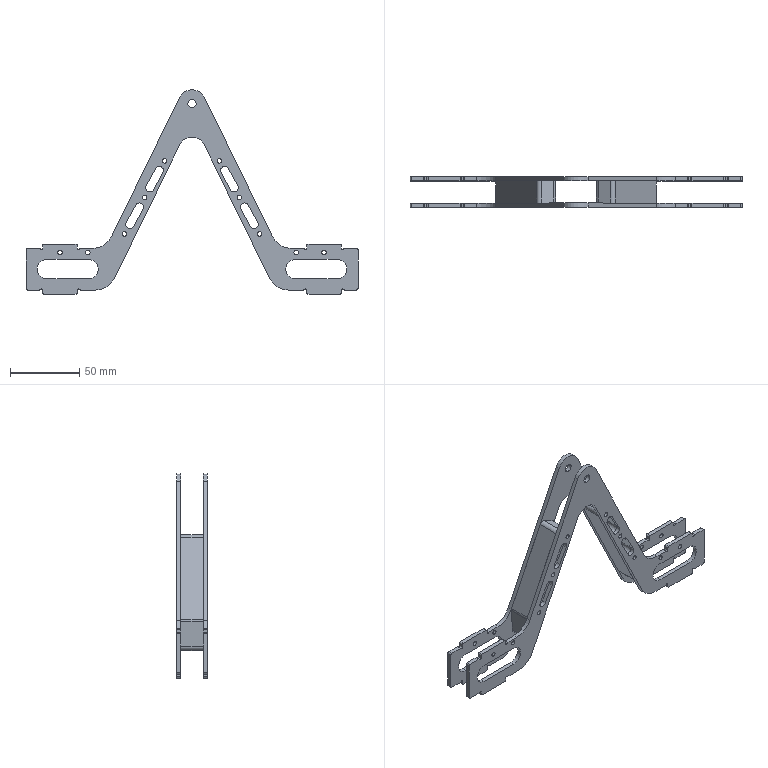Part | SolidWorks | features ICE 5, Extrusion 1, Fillet 1, MirrorSolid 1 | 4 solids | 286 faces | box 239 x 22 x 147.217 mm | volume 68653 mm3 | cylinder 186 | plane 100 | commonest cylinder face diameters 3.2 x52 6 x50 2 x40 1.5 x24 14 x8 30 x8